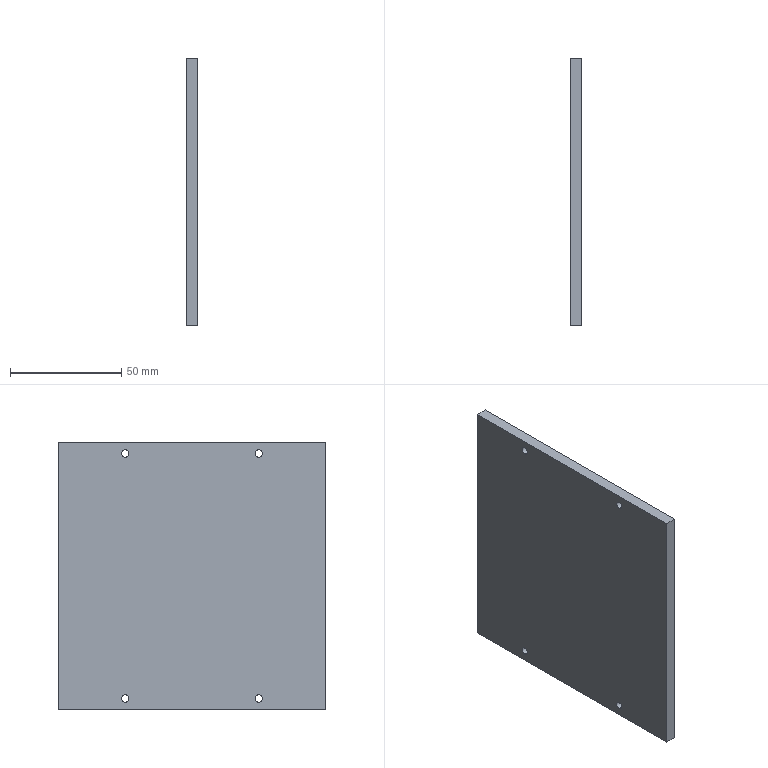Part | NX | 1 solid | 14 faces | box 5 x 120 x 120 mm | volume 71829 mm3 | cylinder 8 | plane 6 | commonest cylinder face diameters 3.3 x8
STEP:
#1=CARTESIAN_POINT('',(0.,-30.,56.65));
#2=VERTEX_POINT('',#1);
#3=CARTESIAN_POINT('',(0.,-30.,53.35));
#4=VERTEX_POINT('',#3);
#5=CARTESIAN_POINT('',(0.,-30.,55.));
#6=DIRECTION('',(1.,0.,0.));
#7=DIRECTION('',(0.,0.,-1.));
#8=AXIS2_PLACEMENT_3D('',#5,#6,#7);
#9=CIRCLE('',#8,1.65);
#10=EDGE_CURVE('',#2,#4,#9,.T.);
#11=ORIENTED_EDGE('',*,*,#10,.F.);
#12=CARTESIAN_POINT('',(5.,-30.,56.65));
#13=VERTEX_POINT('',#12);
#14=CARTESIAN_POINT('',(5.,-30.,56.65));
#15=DIRECTION('',(-1.,0.,0.));
#16=VECTOR('',#15,1.);
#17=LINE('',#14,#16);
#18=EDGE_CURVE('',#13,#2,#17,.T.);
#19=ORIENTED_EDGE('',*,*,#18,.F.);
#20=CARTESIAN_POINT('',(5.,-30.,53.35));
#21=VERTEX_POINT('',#20);
#22=CARTESIAN_POINT('',(5.,-30.,55.));
#23=DIRECTION('',(1.,0.,0.));
#24=DIRECTION('',(0.,0.,-1.));
#25=AXIS2_PLACEMENT_3D('',#22,#23,#24);
#26=CIRCLE('',#25,1.65);
#27=EDGE_CURVE('',#13,#21,#26,.T.);
#28=ORIENTED_EDGE('',*,*,#27,.T.);
#29=CARTESIAN_POINT('',(5.,-30.,53.35));
#30=DIRECTION('',(-1.,0.,0.));
#31=VECTOR('',#30,1.);
#32=LINE('',#29,#31);
#33=EDGE_CURVE('',#21,#4,#32,.T.);
#34=ORIENTED_EDGE('',*,*,#33,.T.);
#35=EDGE_LOOP('',(#11,#19,#28,#34));
#36=FACE_OUTER_BOUND('',#35,.T.);
#37=CARTESIAN_POINT('',(5.,-30.,55.));
#38=DIRECTION('',(1.,0.,0.));
#39=DIRECTION('',(0.,0.,-1.));
#40=AXIS2_PLACEMENT_3D('',#37,#38,#39);
#41=CYLINDRICAL_SURFACE('',#40,1.65);
#42=ADVANCED_FACE('',(#36),#41,.F.);
#43=CARTESIAN_POINT('',(0.,30.,56.65));
#44=VERTEX_POINT('',#43);
#45=CARTESIAN_POINT('',(0.,30.,53.35));
#46=VERTEX_POINT('',#45);
#47=CARTESIAN_POINT('',(0.,30.,55.));
#48=DIRECTION('',(1.,0.,0.));
#49=DIRECTION('',(0.,0.,-1.));
#50=AXIS2_PLACEMENT_3D('',#47,#48,#49);
#51=CIRCLE('',#50,1.65);
#52=EDGE_CURVE('',#44,#46,#51,.T.);
#53=ORIENTED_EDGE('',*,*,#52,.F.);
#54=CARTESIAN_POINT('',(5.,30.,56.65));
#55=VERTEX_POINT('',#54);
#56=CARTESIAN_POINT('',(5.,30.,56.65));
#57=DIRECTION('',(-1.,0.,0.));
#58=VECTOR('',#57,1.);
#59=LINE('',#56,#58);
#60=EDGE_CURVE('',#55,#44,#59,.T.);
#61=ORIENTED_EDGE('',*,*,#60,.F.);
#62=CARTESIAN_POINT('',(5.,30.,53.35));
#63=VERTEX_POINT('',#62);
#64=CARTESIAN_POINT('',(5.,30.,55.));
#65=DIRECTION('',(1.,0.,0.));
#66=DIRECTION('',(0.,0.,-1.));
#67=AXIS2_PLACEMENT_3D('',#64,#65,#66);
#68=CIRCLE('',#67,1.65);
#69=EDGE_CURVE('',#55,#63,#68,.T.);
#70=ORIENTED_EDGE('',*,*,#69,.T.);
#71=CARTESIAN_POINT('',(5.,30.,53.35));
#72=DIRECTION('',(-1.,0.,0.));
#73=VECTOR('',#72,1.);
#74=LINE('',#71,#73);
#75=EDGE_CURVE('',#63,#46,#74,.T.);
#76=ORIENTED_EDGE('',*,*,#75,.T.);
#77=EDGE_LOOP('',(#53,#61,#70,#76));
#78=FACE_OUTER_BOUND('',#77,.T.);
#79=CARTESIAN_POINT('',(5.,30.,55.));
#80=DIRECTION('',(1.,0.,0.));
#81=DIRECTION('',(0.,0.,-1.));
#82=AXIS2_PLACEMENT_3D('',#79,#80,#81);
#83=CYLINDRICAL_SURFACE('',#82,1.65);
#84=ADVANCED_FACE('',(#78),#83,.F.);
#85=CARTESIAN_POINT('',(0.,-30.,-53.35));
#86=VERTEX_POINT('',#85);
#87=CARTESIAN_POINT('',(0.,-30.,-56.65));
#88=VERTEX_POINT('',#87);
#89=CARTESIAN_POINT('',(0.,-30.,-55.));
#90=DIRECTION('',(1.,0.,0.));
#91=DIRECTION('',(0.,0.,-1.));
#92=AXIS2_PLACEMENT_3D('',#89,#90,#91);
#93=CIRCLE('',#92,1.65);
#94=EDGE_CURVE('',#86,#88,#93,.T.);
#95=ORIENTED_EDGE('',*,*,#94,.F.);
#96=CARTESIAN_POINT('',(5.,-30.,-53.35));
#97=VERTEX_POINT('',#96);
#98=CARTESIAN_POINT('',(5.,-30.,-53.35));
#99=DIRECTION('',(-1.,0.,0.));
#100=VECTOR('',#99,1.);
#101=LINE('',#98,#100);
#102=EDGE_CURVE('',#97,#86,#101,.T.);
#103=ORIENTED_EDGE('',*,*,#102,.F.);
#104=CARTESIAN_POINT('',(5.,-30.,-56.65));
#105=VERTEX_POINT('',#104);
#106=CARTESIAN_POINT('',(5.,-30.,-55.));
#107=DIRECTION('',(1.,0.,0.));
#108=DIRECTION('',(0.,0.,-1.));
#109=AXIS2_PLACEMENT_3D('',#106,#107,#108);
#110=CIRCLE('',#109,1.65);
#111=EDGE_CURVE('',#97,#105,#110,.T.);
#112=ORIENTED_EDGE('',*,*,#111,.T.);
#113=CARTESIAN_POINT('',(5.,-30.,-56.65));
#114=DIRECTION('',(-1.,0.,0.));
#115=VECTOR('',#114,1.);
#116=LINE('',#113,#115);
#117=EDGE_CURVE('',#105,#88,#116,.T.);
#118=ORIENTED_EDGE('',*,*,#117,.T.);
#119=EDGE_LOOP('',(#95,#103,#112,#118));
#120=FACE_OUTER_BOUND('',#119,.T.);
#121=CARTESIAN_POINT('',(5.,-30.,-55.));
#122=DIRECTION('',(1.,0.,0.));
#123=DIRECTION('',(0.,0.,-1.));
#124=AXIS2_PLACEMENT_3D('',#121,#122,#123);
#125=CYLINDRICAL_SURFACE('',#124,1.65);
#126=ADVANCED_FACE('',(#120),#125,.F.);
#127=CARTESIAN_POINT('',(0.,30.,-53.35));
#128=VERTEX_POINT('',#127);
#129=CARTESIAN_POINT('',(0.,30.,-56.65));
#130=VERTEX_POINT('',#129);
#131=CARTESIAN_POINT('',(0.,30.,-55.));
#132=DIRECTION('',(1.,0.,0.));
#133=DIRECTION('',(0.,0.,-1.));
#134=AXIS2_PLACEMENT_3D('',#131,#132,#133);
#135=CIRCLE('',#134,1.65);
#136=EDGE_CURVE('',#128,#130,#135,.T.);
#137=ORIENTED_EDGE('',*,*,#136,.F.);
#138=CARTESIAN_POINT('',(5.,30.,-53.35));
#139=VERTEX_POINT('',#138);
#140=CARTESIAN_POINT('',(5.,30.,-53.35));
#141=DIRECTION('',(-1.,0.,0.));
#142=VECTOR('',#141,1.);
#143=LINE('',#140,#142);
#144=EDGE_CURVE('',#139,#128,#143,.T.);
#145=ORIENTED_EDGE('',*,*,#144,.F.);
#146=CARTESIAN_POINT('',(5.,30.,-56.65));
#147=VERTEX_POINT('',#146);
#148=CARTESIAN_POINT('',(5.,30.,-55.));
#149=DIRECTION('',(1.,0.,0.));
#150=DIRECTION('',(0.,0.,-1.));
#151=AXIS2_PLACEMENT_3D('',#148,#149,#150);
#152=CIRCLE('',#151,1.65);
#153=EDGE_CURVE('',#139,#147,#152,.T.);
#154=ORIENTED_EDGE('',*,*,#153,.T.);
#155=CARTESIAN_POINT('',(5.,30.,-56.65));
#156=DIRECTION('',(-1.,0.,0.));
#157=VECTOR('',#156,1.);
#158=LINE('',#155,#157);
#159=EDGE_CURVE('',#147,#130,#158,.T.);
#160=ORIENTED_EDGE('',*,*,#159,.T.);
#161=EDGE_LOOP('',(#137,#145,#154,#160));
#162=FACE_OUTER_BOUND('',#161,.T.);
#163=CARTESIAN_POINT('',(5.,30.,-55.));
#164=DIRECTION('',(1.,0.,0.));
#165=DIRECTION('',(0.,0.,-1.));
#166=AXIS2_PLACEMENT_3D('',#163,#164,#165);
#167=CYLINDRICAL_SURFACE('',#166,1.65);
#168=ADVANCED_FACE('',(#162),#167,.F.);
#169=CARTESIAN_POINT('',(0.,-60.,-60.));
#170=VERTEX_POINT('',#169);
#171=CARTESIAN_POINT('',(0.,60.,-60.));
#172=VERTEX_POINT('',#171);
#173=CARTESIAN_POINT('',(0.,60.,-60.));
#174=DIRECTION('',(0.,1.,0.));
#175=VECTOR('',#174,1.);
#176=LINE('',#173,#175);
#177=EDGE_CURVE('',#170,#172,#176,.T.);
#178=ORIENTED_EDGE('',*,*,#177,.T.);
#179=CARTESIAN_POINT('',(5.,60.,-60.));
#180=VERTEX_POINT('',#179);
#181=CARTESIAN_POINT('',(5.,60.,-60.));
#182=DIRECTION('',(-1.,0.,0.));
#183=VECTOR('',#182,1.);
#184=LINE('',#181,#183);
#185=EDGE_CURVE('',#180,#172,#184,.T.);
#186=ORIENTED_EDGE('',*,*,#185,.F.);
#187=CARTESIAN_POINT('',(5.,-60.,-60.));
#188=VERTEX_POINT('',#187);
#189=CARTESIAN_POINT('',(5.,60.,-60.));
#190=DIRECTION('',(0.,1.,0.));
#191=VECTOR('',#190,1.);
#192=LINE('',#189,#191);
#193=EDGE_CURVE('',#188,#180,#192,.T.);
#194=ORIENTED_EDGE('',*,*,#193,.F.);
#195=CARTESIAN_POINT('',(5.,-60.,-60.));
#196=DIRECTION('',(-1.,0.,0.));
#197=VECTOR('',#196,1.);
#198=LINE('',#195,#197);
#199=EDGE_CURVE('',#188,#170,#198,.T.);
#200=ORIENTED_EDGE('',*,*,#199,.T.);
#201=EDGE_LOOP('',(#178,#186,#194,#200));
#202=FACE_OUTER_BOUND('',#201,.T.);
#203=CARTESIAN_POINT('',(5.,60.,-60.));
#204=DIRECTION('',(0.,0.,1.));
#205=DIRECTION('',(0.,-1.,0.));
#206=AXIS2_PLACEMENT_3D('',#203,#204,#205);
#207=PLANE('',#206);
#208=ADVANCED_FACE('',(#202),#207,.F.);
#209=CARTESIAN_POINT('',(0.,60.,60.));
#210=VERTEX_POINT('',#209);
#211=CARTESIAN_POINT('',(0.,60.,60.));
#212=DIRECTION('',(0.,0.,1.));
#213=VECTOR('',#212,1.);
#214=LINE('',#211,#213);
#215=EDGE_CURVE('',#172,#210,#214,.T.);
#216=ORIENTED_EDGE('',*,*,#215,.T.);
#217=CARTESIAN_POINT('',(5.,60.,60.));
#218=VERTEX_POINT('',#217);
#219=CARTESIAN_POINT('',(5.,60.,60.));
#220=DIRECTION('',(-1.,0.,0.));
#221=VECTOR('',#220,1.);
#222=LINE('',#219,#221);
#223=EDGE_CURVE('',#218,#210,#222,.T.);
#224=ORIENTED_EDGE('',*,*,#223,.F.);
#225=CARTESIAN_POINT('',(5.,60.,60.));
#226=DIRECTION('',(0.,0.,1.));
#227=VECTOR('',#226,1.);
#228=LINE('',#225,#227);
#229=EDGE_CURVE('',#180,#218,#228,.T.);
#230=ORIENTED_EDGE('',*,*,#229,.F.);
#231=ORIENTED_EDGE('',*,*,#185,.T.);
#232=EDGE_LOOP('',(#216,#224,#230,#231));
#233=FACE_OUTER_BOUND('',#232,.T.);
#234=CARTESIAN_POINT('',(5.,60.,60.));
#235=DIRECTION('',(0.,-1.,0.));
#236=DIRECTION('',(0.,0.,-1.));
#237=AXIS2_PLACEMENT_3D('',#234,#235,#236);
#238=PLANE('',#237);
#239=ADVANCED_FACE('',(#233),#238,.F.);
#240=CARTESIAN_POINT('',(0.,-60.,60.));
#241=VERTEX_POINT('',#240);
#242=CARTESIAN_POINT('',(0.,60.,60.));
#243=DIRECTION('',(0.,-1.,0.));
#244=VECTOR('',#243,1.);
#245=LINE('',#242,#244);
#246=EDGE_CURVE('',#210,#241,#245,.T.);
#247=ORIENTED_EDGE('',*,*,#246,.T.);
#248=CARTESIAN_POINT('',(5.,-60.,60.));
#249=VERTEX_POINT('',#248);
#250=CARTESIAN_POINT('',(5.,-60.,60.));
#251=DIRECTION('',(-1.,0.,0.));
#252=VECTOR('',#251,1.);
#253=LINE('',#250,#252);
#254=EDGE_CURVE('',#249,#241,#253,.T.);
#255=ORIENTED_EDGE('',*,*,#254,.F.);
#256=CARTESIAN_POINT('',(5.,60.,60.));
#257=DIRECTION('',(0.,-1.,0.));
#258=VECTOR('',#257,1.);
#259=LINE('',#256,#258);
#260=EDGE_CURVE('',#218,#249,#259,.T.);
#261=ORIENTED_EDGE('',*,*,#260,.F.);
#262=ORIENTED_EDGE('',*,*,#223,.T.);
#263=EDGE_LOOP('',(#247,#255,#261,#262));
#264=FACE_OUTER_BOUND('',#263,.T.);
#265=CARTESIAN_POINT('',(5.,60.,60.));
#266=DIRECTION('',(0.,0.,-1.));
#267=DIRECTION('',(0.,1.,0.));
#268=AXIS2_PLACEMENT_3D('',#265,#266,#267);
#269=PLANE('',#268);
#270=ADVANCED_FACE('',(#264),#269,.F.);
#271=CARTESIAN_POINT('',(0.,-60.,60.));
#272=DIRECTION('',(0.,0.,-1.));
#273=VECTOR('',#272,1.);
#274=LINE('',#271,#273);
#275=EDGE_CURVE('',#241,#170,#274,.T.);
#276=ORIENTED_EDGE('',*,*,#275,.T.);
#277=ORIENTED_EDGE('',*,*,#199,.F.);
#278=CARTESIAN_POINT('',(5.,-60.,60.));
#279=DIRECTION('',(0.,0.,-1.));
#280=VECTOR('',#279,1.);
#281=LINE('',#278,#280);
#282=EDGE_CURVE('',#249,#188,#281,.T.);
#283=ORIENTED_EDGE('',*,*,#282,.F.);
#284=ORIENTED_EDGE('',*,*,#254,.T.);
#285=EDGE_LOOP('',(#276,#277,#283,#284));
#286=FACE_OUTER_BOUND('',#285,.T.);
#287=CARTESIAN_POINT('',(5.,-60.,60.));
#288=DIRECTION('',(0.,1.,0.));
#289=DIRECTION('',(0.,0.,1.));
#290=AXIS2_PLACEMENT_3D('',#287,#288,#289);
#291=PLANE('',#290);
#292=ADVANCED_FACE('',(#286),#291,.F.);
#293=CARTESIAN_POINT('',(5.,-30.,55.));
#294=DIRECTION('',(1.,0.,0.));
#295=DIRECTION('',(0.,0.,-1.));
#296=AXIS2_PLACEMENT_3D('',#293,#294,#295);
#297=CIRCLE('',#296,1.65);
#298=EDGE_CURVE('',#21,#13,#297,.T.);
#299=ORIENTED_EDGE('',*,*,#298,.F.);
#300=ORIENTED_EDGE('',*,*,#27,.F.);
#301=EDGE_LOOP('',(#299,#300));
#302=FACE_BOUND('',#301,.T.);
#303=CARTESIAN_POINT('',(5.,30.,55.));
#304=DIRECTION('',(1.,0.,0.));
#305=DIRECTION('',(0.,0.,-1.));
#306=AXIS2_PLACEMENT_3D('',#303,#304,#305);
#307=CIRCLE('',#306,1.65);
#308=EDGE_CURVE('',#63,#55,#307,.T.);
#309=ORIENTED_EDGE('',*,*,#308,.F.);
#310=ORIENTED_EDGE('',*,*,#69,.F.);
#311=EDGE_LOOP('',(#309,#310));
#312=FACE_BOUND('',#311,.T.);
#313=CARTESIAN_POINT('',(5.,-30.,-55.));
#314=DIRECTION('',(1.,0.,0.));
#315=DIRECTION('',(0.,0.,-1.));
#316=AXIS2_PLACEMENT_3D('',#313,#314,#315);
#317=CIRCLE('',#316,1.65);
#318=EDGE_CURVE('',#105,#97,#317,.T.);
#319=ORIENTED_EDGE('',*,*,#318,.F.);
#320=ORIENTED_EDGE('',*,*,#111,.F.);
#321=EDGE_LOOP('',(#319,#320));
#322=FACE_BOUND('',#321,.T.);
#323=CARTESIAN_POINT('',(5.,30.,-55.));
#324=DIRECTION('',(1.,0.,0.));
#325=DIRECTION('',(0.,0.,-1.));
#326=AXIS2_PLACEMENT_3D('',#323,#324,#325);
#327=CIRCLE('',#326,1.65);
#328=EDGE_CURVE('',#147,#139,#327,.T.);
#329=ORIENTED_EDGE('',*,*,#328,.F.);
#330=ORIENTED_EDGE('',*,*,#153,.F.);
#331=EDGE_LOOP('',(#329,#330));
#332=FACE_BOUND('',#331,.T.);
#333=ORIENTED_EDGE('',*,*,#193,.T.);
#334=ORIENTED_EDGE('',*,*,#229,.T.);
#335=ORIENTED_EDGE('',*,*,#260,.T.);
#336=ORIENTED_EDGE('',*,*,#282,.T.);
#337=EDGE_LOOP('',(#333,#334,#335,#336));
#338=FACE_BOUND('',#337,.T.);
#339=CARTESIAN_POINT('',(5.,-60.,-60.));
#340=DIRECTION('',(1.,0.,0.));
#341=DIRECTION('',(0.,0.,-1.));
#342=AXIS2_PLACEMENT_3D('',#339,#340,#341);
#343=PLANE('',#342);
#344=ADVANCED_FACE('',(#302,#312,#322,#332,#338),#343,.T.);
#345=CARTESIAN_POINT('',(0.,-30.,55.));
#346=DIRECTION('',(1.,0.,0.));
#347=DIRECTION('',(0.,0.,-1.));
#348=AXIS2_PLACEMENT_3D('',#345,#346,#347);
#349=CIRCLE('',#348,1.65);
#350=EDGE_CURVE('',#4,#2,#349,.T.);
#351=ORIENTED_EDGE('',*,*,#350,.T.);
#352=ORIENTED_EDGE('',*,*,#10,.T.);
#353=EDGE_LOOP('',(#351,#352));
#354=FACE_BOUND('',#353,.T.);
#355=CARTESIAN_POINT('',(0.,30.,55.));
#356=DIRECTION('',(1.,0.,0.));
#357=DIRECTION('',(0.,0.,-1.));
#358=AXIS2_PLACEMENT_3D('',#355,#356,#357);
#359=CIRCLE('',#358,1.65);
#360=EDGE_CURVE('',#46,#44,#359,.T.);
#361=ORIENTED_EDGE('',*,*,#360,.T.);
#362=ORIENTED_EDGE('',*,*,#52,.T.);
#363=EDGE_LOOP('',(#361,#362));
#364=FACE_BOUND('',#363,.T.);
#365=CARTESIAN_POINT('',(0.,-30.,-55.));
#366=DIRECTION('',(1.,0.,0.));
#367=DIRECTION('',(0.,0.,-1.));
#368=AXIS2_PLACEMENT_3D('',#365,#366,#367);
#369=CIRCLE('',#368,1.65);
#370=EDGE_CURVE('',#88,#86,#369,.T.);
#371=ORIENTED_EDGE('',*,*,#370,.T.);
#372=ORIENTED_EDGE('',*,*,#94,.T.);
#373=EDGE_LOOP('',(#371,#372));
#374=FACE_BOUND('',#373,.T.);
#375=CARTESIAN_POINT('',(0.,30.,-55.));
#376=DIRECTION('',(1.,0.,0.));
#377=DIRECTION('',(0.,0.,-1.));
#378=AXIS2_PLACEMENT_3D('',#375,#376,#377);
#379=CIRCLE('',#378,1.65);
#380=EDGE_CURVE('',#130,#128,#379,.T.);
#381=ORIENTED_EDGE('',*,*,#380,.T.);
#382=ORIENTED_EDGE('',*,*,#136,.T.);
#383=EDGE_LOOP('',(#381,#382));
#384=FACE_BOUND('',#383,.T.);
#385=ORIENTED_EDGE('',*,*,#177,.F.);
#386=ORIENTED_EDGE('',*,*,#275,.F.);
#387=ORIENTED_EDGE('',*,*,#246,.F.);
#388=ORIENTED_EDGE('',*,*,#215,.F.);
#389=EDGE_LOOP('',(#385,#386,#387,#388));
#390=FACE_BOUND('',#389,.T.);
#391=CARTESIAN_POINT('',(0.,-60.,-60.));
#392=DIRECTION('',(1.,0.,0.));
#393=DIRECTION('',(0.,0.,-1.));
#394=AXIS2_PLACEMENT_3D('',#391,#392,#393);
#395=PLANE('',#394);
#396=ADVANCED_FACE('',(#354,#364,#374,#384,#390),#395,.F.);
#397=ORIENTED_EDGE('',*,*,#144,.T.);
#398=ORIENTED_EDGE('',*,*,#380,.F.);
#399=ORIENTED_EDGE('',*,*,#159,.F.);
#400=ORIENTED_EDGE('',*,*,#328,.T.);
#401=EDGE_LOOP('',(#397,#398,#399,#400));
#402=FACE_OUTER_BOUND('',#401,.T.);
#403=CARTESIAN_POINT('',(5.,30.,-55.));
#404=DIRECTION('',(1.,0.,0.));
#405=DIRECTION('',(0.,0.,-1.));
#406=AXIS2_PLACEMENT_3D('',#403,#404,#405);
#407=CYLINDRICAL_SURFACE('',#406,1.65);
#408=ADVANCED_FACE('',(#402),#407,.F.);
#409=ORIENTED_EDGE('',*,*,#102,.T.);
#410=ORIENTED_EDGE('',*,*,#370,.F.);
#411=ORIENTED_EDGE('',*,*,#117,.F.);
#412=ORIENTED_EDGE('',*,*,#318,.T.);
#413=EDGE_LOOP('',(#409,#410,#411,#412));
#414=FACE_OUTER_BOUND('',#413,.T.);
#415=CARTESIAN_POINT('',(5.,-30.,-55.));
#416=DIRECTION('',(1.,0.,0.));
#417=DIRECTION('',(0.,0.,-1.));
#418=AXIS2_PLACEMENT_3D('',#415,#416,#417);
#419=CYLINDRICAL_SURFACE('',#418,1.65);
#420=ADVANCED_FACE('',(#414),#419,.F.);
#421=ORIENTED_EDGE('',*,*,#60,.T.);
#422=ORIENTED_EDGE('',*,*,#360,.F.);
#423=ORIENTED_EDGE('',*,*,#75,.F.);
#424=ORIENTED_EDGE('',*,*,#308,.T.);
#425=EDGE_LOOP('',(#421,#422,#423,#424));
#426=FACE_OUTER_BOUND('',#425,.T.);
#427=CARTESIAN_POINT('',(5.,30.,55.));
#428=DIRECTION('',(1.,0.,0.));
#429=DIRECTION('',(0.,0.,-1.));
#430=AXIS2_PLACEMENT_3D('',#427,#428,#429);
#431=CYLINDRICAL_SURFACE('',#430,1.65);
#432=ADVANCED_FACE('',(#426),#431,.F.);
#433=ORIENTED_EDGE('',*,*,#18,.T.);
#434=ORIENTED_EDGE('',*,*,#350,.F.);
#435=ORIENTED_EDGE('',*,*,#33,.F.);
#436=ORIENTED_EDGE('',*,*,#298,.T.);
#437=EDGE_LOOP('',(#433,#434,#435,#436));
#438=FACE_OUTER_BOUND('',#437,.T.);
#439=CARTESIAN_POINT('',(5.,-30.,55.));
#440=DIRECTION('',(1.,0.,0.));
#441=DIRECTION('',(0.,0.,-1.));
#442=AXIS2_PLACEMENT_3D('',#439,#440,#441);
#443=CYLINDRICAL_SURFACE('',#442,1.65);
#444=ADVANCED_FACE('',(#438),#443,.F.);
#445=CLOSED_SHELL('',(#42,#84,#126,#168,#208,#239,#270,#292,#344,#396,#408,#420,#432,#444));
#446=MANIFOLD_SOLID_BREP('',#445);
#447=(LENGTH_UNIT()NAMED_UNIT(*)SI_UNIT(.MILLI.,.METRE.));
#448=UNCERTAINTY_MEASURE_WITH_UNIT(LENGTH_MEASURE(0.00002),#447,'','');
#449=(NAMED_UNIT(*)PLANE_ANGLE_UNIT()SI_UNIT($,.RADIAN.));
#450=PLANE_ANGLE_MEASURE_WITH_UNIT(PLANE_ANGLE_MEASURE(0.01745),#449);
#451=DIMENSIONAL_EXPONENTS(0.,0.,0.,0.,0.,0.,0.);
#452=(CONVERSION_BASED_UNIT('DEGREE',#450)NAMED_UNIT(#451)PLANE_ANGLE_UNIT());
#453=(NAMED_UNIT(*)SI_UNIT($,.STERADIAN.)SOLID_ANGLE_UNIT());
#454=(GEOMETRIC_REPRESENTATION_CONTEXT(3)GLOBAL_UNCERTAINTY_ASSIGNED_CONTEXT((#448))GLOBAL_UNIT_ASSIGNED_CONTEXT((#447,#452,#453))REPRESENTATION_CONTEXT('',''));
#455=ADVANCED_BREP_SHAPE_REPRESENTATION('',(#446),#454);